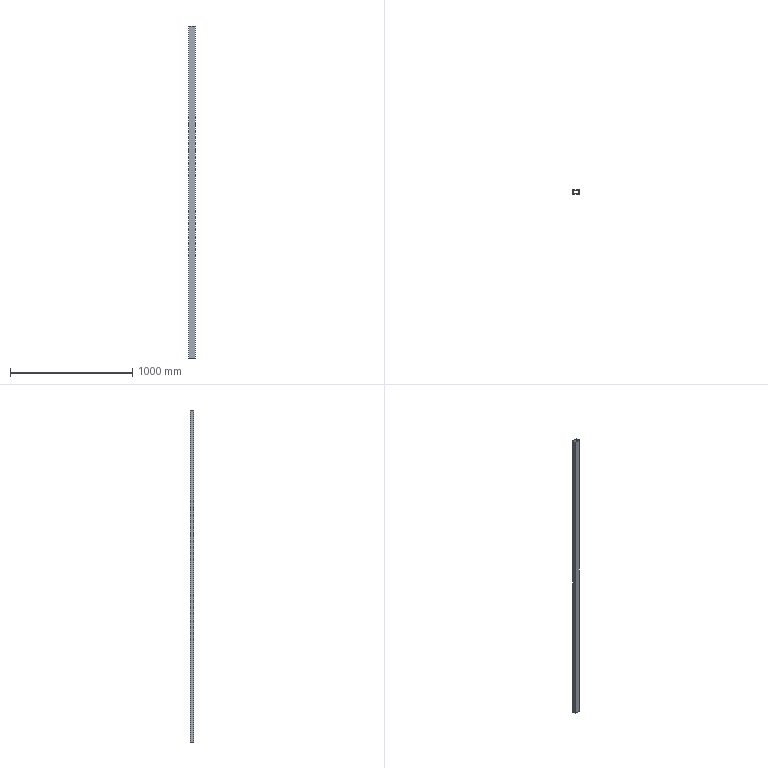Part | SolidWorks | features BaseBody 1 | 1 solid | 10 faces | box 50 x 30 x 2720 mm | volume 628320 mm3 | plane 10
STEP:
#1=CARTESIAN_POINT('',(-25.,15.,2720.));
#2=VERTEX_POINT('',#1);
#3=CARTESIAN_POINT('',(-25.,15.,0.));
#4=VERTEX_POINT('',#3);
#5=CARTESIAN_POINT('',(-25.,15.,2720.));
#6=DIRECTION('',(0.,0.,-1.));
#7=VECTOR('',#6,1000.);
#8=LINE('',#5,#7);
#9=EDGE_CURVE('',#2,#4,#8,.T.);
#10=ORIENTED_EDGE('',*,*,#9,.F.);
#11=CARTESIAN_POINT('',(25.,15.,2720.));
#12=VERTEX_POINT('',#11);
#13=CARTESIAN_POINT('',(-25.,15.,2720.));
#14=DIRECTION('',(-1.,0.,0.));
#15=VECTOR('',#14,1000.);
#16=LINE('',#13,#15);
#17=EDGE_CURVE('',#12,#2,#16,.T.);
#18=ORIENTED_EDGE('',*,*,#17,.F.);
#19=CARTESIAN_POINT('',(25.,15.,0.));
#20=VERTEX_POINT('',#19);
#21=CARTESIAN_POINT('',(25.,15.,2720.));
#22=DIRECTION('',(0.,0.,1.));
#23=VECTOR('',#22,1000.);
#24=LINE('',#21,#23);
#25=EDGE_CURVE('',#20,#12,#24,.T.);
#26=ORIENTED_EDGE('',*,*,#25,.F.);
#27=CARTESIAN_POINT('',(-25.,15.,0.));
#28=DIRECTION('',(1.,0.,0.));
#29=VECTOR('',#28,1000.);
#30=LINE('',#27,#29);
#31=EDGE_CURVE('',#4,#20,#30,.T.);
#32=ORIENTED_EDGE('',*,*,#31,.F.);
#33=EDGE_LOOP('',(#10,#18,#26,#32));
#34=FACE_OUTER_BOUND('',#33,.T.);
#35=CARTESIAN_POINT('',(-25.,15.,2720.));
#36=DIRECTION('',(0.,-1.,0.));
#37=DIRECTION('',(0.,0.,-1.));
#38=AXIS2_PLACEMENT_3D('',#35,#36,#37);
#39=PLANE('',#38);
#40=ADVANCED_FACE('',(#34),#39,.F.);
#41=CARTESIAN_POINT('',(23.5,-13.5,0.));
#42=VERTEX_POINT('',#41);
#43=CARTESIAN_POINT('',(-23.5,-13.5,0.));
#44=VERTEX_POINT('',#43);
#45=CARTESIAN_POINT('',(0.,-13.5,0.));
#46=DIRECTION('',(-1.,0.,0.));
#47=VECTOR('',#46,1000.);
#48=LINE('',#45,#47);
#49=EDGE_CURVE('',#42,#44,#48,.T.);
#50=ORIENTED_EDGE('',*,*,#49,.F.);
#51=CARTESIAN_POINT('',(23.5,13.5,0.));
#52=VERTEX_POINT('',#51);
#53=CARTESIAN_POINT('',(23.5,0.,0.));
#54=DIRECTION('',(0.,-1.,0.));
#55=VECTOR('',#54,1000.);
#56=LINE('',#53,#55);
#57=EDGE_CURVE('',#52,#42,#56,.T.);
#58=ORIENTED_EDGE('',*,*,#57,.F.);
#59=CARTESIAN_POINT('',(-23.5,13.5,0.));
#60=VERTEX_POINT('',#59);
#61=CARTESIAN_POINT('',(0.,13.5,0.));
#62=DIRECTION('',(1.,0.,0.));
#63=VECTOR('',#62,1000.);
#64=LINE('',#61,#63);
#65=EDGE_CURVE('',#60,#52,#64,.T.);
#66=ORIENTED_EDGE('',*,*,#65,.F.);
#67=CARTESIAN_POINT('',(-23.5,0.,0.));
#68=DIRECTION('',(0.,1.,0.));
#69=VECTOR('',#68,1000.);
#70=LINE('',#67,#69);
#71=EDGE_CURVE('',#44,#60,#70,.T.);
#72=ORIENTED_EDGE('',*,*,#71,.F.);
#73=EDGE_LOOP('',(#50,#58,#66,#72));
#74=FACE_BOUND('',#73,.T.);
#75=CARTESIAN_POINT('',(-25.,-15.,0.));
#76=VERTEX_POINT('',#75);
#77=CARTESIAN_POINT('',(25.,-15.,0.));
#78=VERTEX_POINT('',#77);
#79=CARTESIAN_POINT('',(0.,-15.,0.));
#80=DIRECTION('',(1.,0.,0.));
#81=VECTOR('',#80,1000.);
#82=LINE('',#79,#81);
#83=EDGE_CURVE('',#76,#78,#82,.T.);
#84=ORIENTED_EDGE('',*,*,#83,.F.);
#85=CARTESIAN_POINT('',(-25.,0.,0.));
#86=DIRECTION('',(0.,-1.,0.));
#87=VECTOR('',#86,1000.);
#88=LINE('',#85,#87);
#89=EDGE_CURVE('',#4,#76,#88,.T.);
#90=ORIENTED_EDGE('',*,*,#89,.F.);
#91=ORIENTED_EDGE('',*,*,#31,.T.);
#92=CARTESIAN_POINT('',(25.,0.,0.));
#93=DIRECTION('',(0.,1.,0.));
#94=VECTOR('',#93,1000.);
#95=LINE('',#92,#94);
#96=EDGE_CURVE('',#78,#20,#95,.T.);
#97=ORIENTED_EDGE('',*,*,#96,.F.);
#98=EDGE_LOOP('',(#84,#90,#91,#97));
#99=FACE_OUTER_BOUND('',#98,.T.);
#100=CARTESIAN_POINT('',(0.,0.,0.));
#101=DIRECTION('',(0.,0.,1.));
#102=DIRECTION('',(1.,0.,0.));
#103=AXIS2_PLACEMENT_3D('',#100,#101,#102);
#104=PLANE('',#103);
#105=ADVANCED_FACE('',(#74,#99),#104,.F.);
#106=CARTESIAN_POINT('',(-25.,-15.,2720.));
#107=VERTEX_POINT('',#106);
#108=CARTESIAN_POINT('',(-25.,-15.,2720.));
#109=DIRECTION('',(0.,0.,-1.));
#110=VECTOR('',#109,1000.);
#111=LINE('',#108,#110);
#112=EDGE_CURVE('',#107,#76,#111,.T.);
#113=ORIENTED_EDGE('',*,*,#112,.F.);
#114=CARTESIAN_POINT('',(-25.,15.,2720.));
#115=DIRECTION('',(0.,-1.,0.));
#116=VECTOR('',#115,1000.);
#117=LINE('',#114,#116);
#118=EDGE_CURVE('',#2,#107,#117,.T.);
#119=ORIENTED_EDGE('',*,*,#118,.F.);
#120=ORIENTED_EDGE('',*,*,#9,.T.);
#121=ORIENTED_EDGE('',*,*,#89,.T.);
#122=EDGE_LOOP('',(#113,#119,#120,#121));
#123=FACE_OUTER_BOUND('',#122,.T.);
#124=CARTESIAN_POINT('',(-25.,15.,2720.));
#125=DIRECTION('',(1.,0.,0.));
#126=DIRECTION('',(0.,1.,0.));
#127=AXIS2_PLACEMENT_3D('',#124,#125,#126);
#128=PLANE('',#127);
#129=ADVANCED_FACE('',(#123),#128,.F.);
#130=CARTESIAN_POINT('',(-23.5,13.5,2720.));
#131=VERTEX_POINT('',#130);
#132=CARTESIAN_POINT('',(23.5,13.5,2720.));
#133=VERTEX_POINT('',#132);
#134=CARTESIAN_POINT('',(0.,13.5,2720.));
#135=DIRECTION('',(1.,0.,0.));
#136=VECTOR('',#135,1000.);
#137=LINE('',#134,#136);
#138=EDGE_CURVE('',#131,#133,#137,.T.);
#139=ORIENTED_EDGE('',*,*,#138,.T.);
#140=CARTESIAN_POINT('',(23.5,-13.5,2720.));
#141=VERTEX_POINT('',#140);
#142=CARTESIAN_POINT('',(23.5,0.,2720.));
#143=DIRECTION('',(0.,-1.,0.));
#144=VECTOR('',#143,1000.);
#145=LINE('',#142,#144);
#146=EDGE_CURVE('',#133,#141,#145,.T.);
#147=ORIENTED_EDGE('',*,*,#146,.T.);
#148=CARTESIAN_POINT('',(-23.5,-13.5,2720.));
#149=VERTEX_POINT('',#148);
#150=CARTESIAN_POINT('',(0.,-13.5,2720.));
#151=DIRECTION('',(-1.,0.,0.));
#152=VECTOR('',#151,1000.);
#153=LINE('',#150,#152);
#154=EDGE_CURVE('',#141,#149,#153,.T.);
#155=ORIENTED_EDGE('',*,*,#154,.T.);
#156=CARTESIAN_POINT('',(-23.5,0.,2720.));
#157=DIRECTION('',(0.,1.,0.));
#158=VECTOR('',#157,1000.);
#159=LINE('',#156,#158);
#160=EDGE_CURVE('',#149,#131,#159,.T.);
#161=ORIENTED_EDGE('',*,*,#160,.T.);
#162=EDGE_LOOP('',(#139,#147,#155,#161));
#163=FACE_BOUND('',#162,.T.);
#164=ORIENTED_EDGE('',*,*,#118,.T.);
#165=CARTESIAN_POINT('',(25.,-15.,2720.));
#166=VERTEX_POINT('',#165);
#167=CARTESIAN_POINT('',(0.,-15.,2720.));
#168=DIRECTION('',(1.,0.,0.));
#169=VECTOR('',#168,1000.);
#170=LINE('',#167,#169);
#171=EDGE_CURVE('',#107,#166,#170,.T.);
#172=ORIENTED_EDGE('',*,*,#171,.T.);
#173=CARTESIAN_POINT('',(25.,0.,2720.));
#174=DIRECTION('',(0.,1.,0.));
#175=VECTOR('',#174,1000.);
#176=LINE('',#173,#175);
#177=EDGE_CURVE('',#166,#12,#176,.T.);
#178=ORIENTED_EDGE('',*,*,#177,.T.);
#179=ORIENTED_EDGE('',*,*,#17,.T.);
#180=EDGE_LOOP('',(#164,#172,#178,#179));
#181=FACE_OUTER_BOUND('',#180,.T.);
#182=CARTESIAN_POINT('',(0.,0.,2720.));
#183=DIRECTION('',(0.,0.,1.));
#184=DIRECTION('',(1.,0.,0.));
#185=AXIS2_PLACEMENT_3D('',#182,#183,#184);
#186=PLANE('',#185);
#187=ADVANCED_FACE('',(#163,#181),#186,.T.);
#188=ORIENTED_EDGE('',*,*,#25,.T.);
#189=ORIENTED_EDGE('',*,*,#177,.F.);
#190=CARTESIAN_POINT('',(25.,-15.,2720.));
#191=DIRECTION('',(0.,0.,1.));
#192=VECTOR('',#191,1000.);
#193=LINE('',#190,#192);
#194=EDGE_CURVE('',#78,#166,#193,.T.);
#195=ORIENTED_EDGE('',*,*,#194,.F.);
#196=ORIENTED_EDGE('',*,*,#96,.T.);
#197=EDGE_LOOP('',(#188,#189,#195,#196));
#198=FACE_OUTER_BOUND('',#197,.T.);
#199=CARTESIAN_POINT('',(25.,15.,2720.));
#200=DIRECTION('',(-1.,0.,0.));
#201=DIRECTION('',(0.,-1.,0.));
#202=AXIS2_PLACEMENT_3D('',#199,#200,#201);
#203=PLANE('',#202);
#204=ADVANCED_FACE('',(#198),#203,.F.);
#205=ORIENTED_EDGE('',*,*,#160,.F.);
#206=CARTESIAN_POINT('',(-23.5,-13.5,2720.));
#207=DIRECTION('',(0.,0.,-1.));
#208=VECTOR('',#207,1000.);
#209=LINE('',#206,#208);
#210=EDGE_CURVE('',#149,#44,#209,.T.);
#211=ORIENTED_EDGE('',*,*,#210,.T.);
#212=ORIENTED_EDGE('',*,*,#71,.T.);
#213=CARTESIAN_POINT('',(-23.5,13.5,2720.));
#214=DIRECTION('',(0.,0.,1.));
#215=VECTOR('',#214,1000.);
#216=LINE('',#213,#215);
#217=EDGE_CURVE('',#60,#131,#216,.T.);
#218=ORIENTED_EDGE('',*,*,#217,.T.);
#219=EDGE_LOOP('',(#205,#211,#212,#218));
#220=FACE_OUTER_BOUND('',#219,.T.);
#221=CARTESIAN_POINT('',(-23.5,13.5,2720.));
#222=DIRECTION('',(1.,0.,0.));
#223=DIRECTION('',(0.,0.,-1.));
#224=AXIS2_PLACEMENT_3D('',#221,#222,#223);
#225=PLANE('',#224);
#226=ADVANCED_FACE('',(#220),#225,.T.);
#227=ORIENTED_EDGE('',*,*,#154,.F.);
#228=CARTESIAN_POINT('',(23.5,-13.5,2720.));
#229=DIRECTION('',(0.,0.,-1.));
#230=VECTOR('',#229,1000.);
#231=LINE('',#228,#230);
#232=EDGE_CURVE('',#141,#42,#231,.T.);
#233=ORIENTED_EDGE('',*,*,#232,.T.);
#234=ORIENTED_EDGE('',*,*,#49,.T.);
#235=ORIENTED_EDGE('',*,*,#210,.F.);
#236=EDGE_LOOP('',(#227,#233,#234,#235));
#237=FACE_OUTER_BOUND('',#236,.T.);
#238=CARTESIAN_POINT('',(23.5,-13.5,2720.));
#239=DIRECTION('',(0.,1.,0.));
#240=DIRECTION('',(0.,0.,1.));
#241=AXIS2_PLACEMENT_3D('',#238,#239,#240);
#242=PLANE('',#241);
#243=ADVANCED_FACE('',(#237),#242,.T.);
#244=ORIENTED_EDGE('',*,*,#146,.F.);
#245=CARTESIAN_POINT('',(23.5,13.5,2720.));
#246=DIRECTION('',(0.,0.,-1.));
#247=VECTOR('',#246,1000.);
#248=LINE('',#245,#247);
#249=EDGE_CURVE('',#133,#52,#248,.T.);
#250=ORIENTED_EDGE('',*,*,#249,.T.);
#251=ORIENTED_EDGE('',*,*,#57,.T.);
#252=ORIENTED_EDGE('',*,*,#232,.F.);
#253=EDGE_LOOP('',(#244,#250,#251,#252));
#254=FACE_OUTER_BOUND('',#253,.T.);
#255=CARTESIAN_POINT('',(23.5,13.5,2720.));
#256=DIRECTION('',(-1.,0.,0.));
#257=DIRECTION('',(0.,0.,1.));
#258=AXIS2_PLACEMENT_3D('',#255,#256,#257);
#259=PLANE('',#258);
#260=ADVANCED_FACE('',(#254),#259,.T.);
#261=ORIENTED_EDGE('',*,*,#138,.F.);
#262=ORIENTED_EDGE('',*,*,#217,.F.);
#263=ORIENTED_EDGE('',*,*,#65,.T.);
#264=ORIENTED_EDGE('',*,*,#249,.F.);
#265=EDGE_LOOP('',(#261,#262,#263,#264));
#266=FACE_OUTER_BOUND('',#265,.T.);
#267=CARTESIAN_POINT('',(23.5,13.5,2720.));
#268=DIRECTION('',(0.,-1.,0.));
#269=DIRECTION('',(0.,0.,-1.));
#270=AXIS2_PLACEMENT_3D('',#267,#268,#269);
#271=PLANE('',#270);
#272=ADVANCED_FACE('',(#266),#271,.T.);
#273=ORIENTED_EDGE('',*,*,#194,.T.);
#274=ORIENTED_EDGE('',*,*,#171,.F.);
#275=ORIENTED_EDGE('',*,*,#112,.T.);
#276=ORIENTED_EDGE('',*,*,#83,.T.);
#277=EDGE_LOOP('',(#273,#274,#275,#276));
#278=FACE_OUTER_BOUND('',#277,.T.);
#279=CARTESIAN_POINT('',(-25.,-15.,2720.));
#280=DIRECTION('',(0.,1.,0.));
#281=DIRECTION('',(0.,0.,1.));
#282=AXIS2_PLACEMENT_3D('',#279,#280,#281);
#283=PLANE('',#282);
#284=ADVANCED_FACE('',(#278),#283,.F.);
#285=CLOSED_SHELL('',(#40,#105,#129,#187,#204,#226,#243,#260,#272,#284));
#286=MANIFOLD_SOLID_BREP('',#285);
#287=CARTESIAN_POINT('',(0.,0.,0.));
#288=DIRECTION('',(0.,0.,1.));
#289=DIRECTION('',(1.,0.,0.));
#290=AXIS2_PLACEMENT_3D('',#287,#288,#289);
#291=(LENGTH_UNIT()NAMED_UNIT(*)SI_UNIT(.MILLI.,.METRE.));
#292=UNCERTAINTY_MEASURE_WITH_UNIT(LENGTH_MEASURE(0.00001),#291,'','');
#293=(NAMED_UNIT(*)PLANE_ANGLE_UNIT()SI_UNIT($,.RADIAN.));
#294=(NAMED_UNIT(*)SI_UNIT($,.STERADIAN.)SOLID_ANGLE_UNIT());
#295=(GEOMETRIC_REPRESENTATION_CONTEXT(3)GLOBAL_UNCERTAINTY_ASSIGNED_CONTEXT((#292))GLOBAL_UNIT_ASSIGNED_CONTEXT((#291,#293,#294))REPRESENTATION_CONTEXT('',''));
#296=ADVANCED_BREP_SHAPE_REPRESENTATION('',(#286,#290),#295);